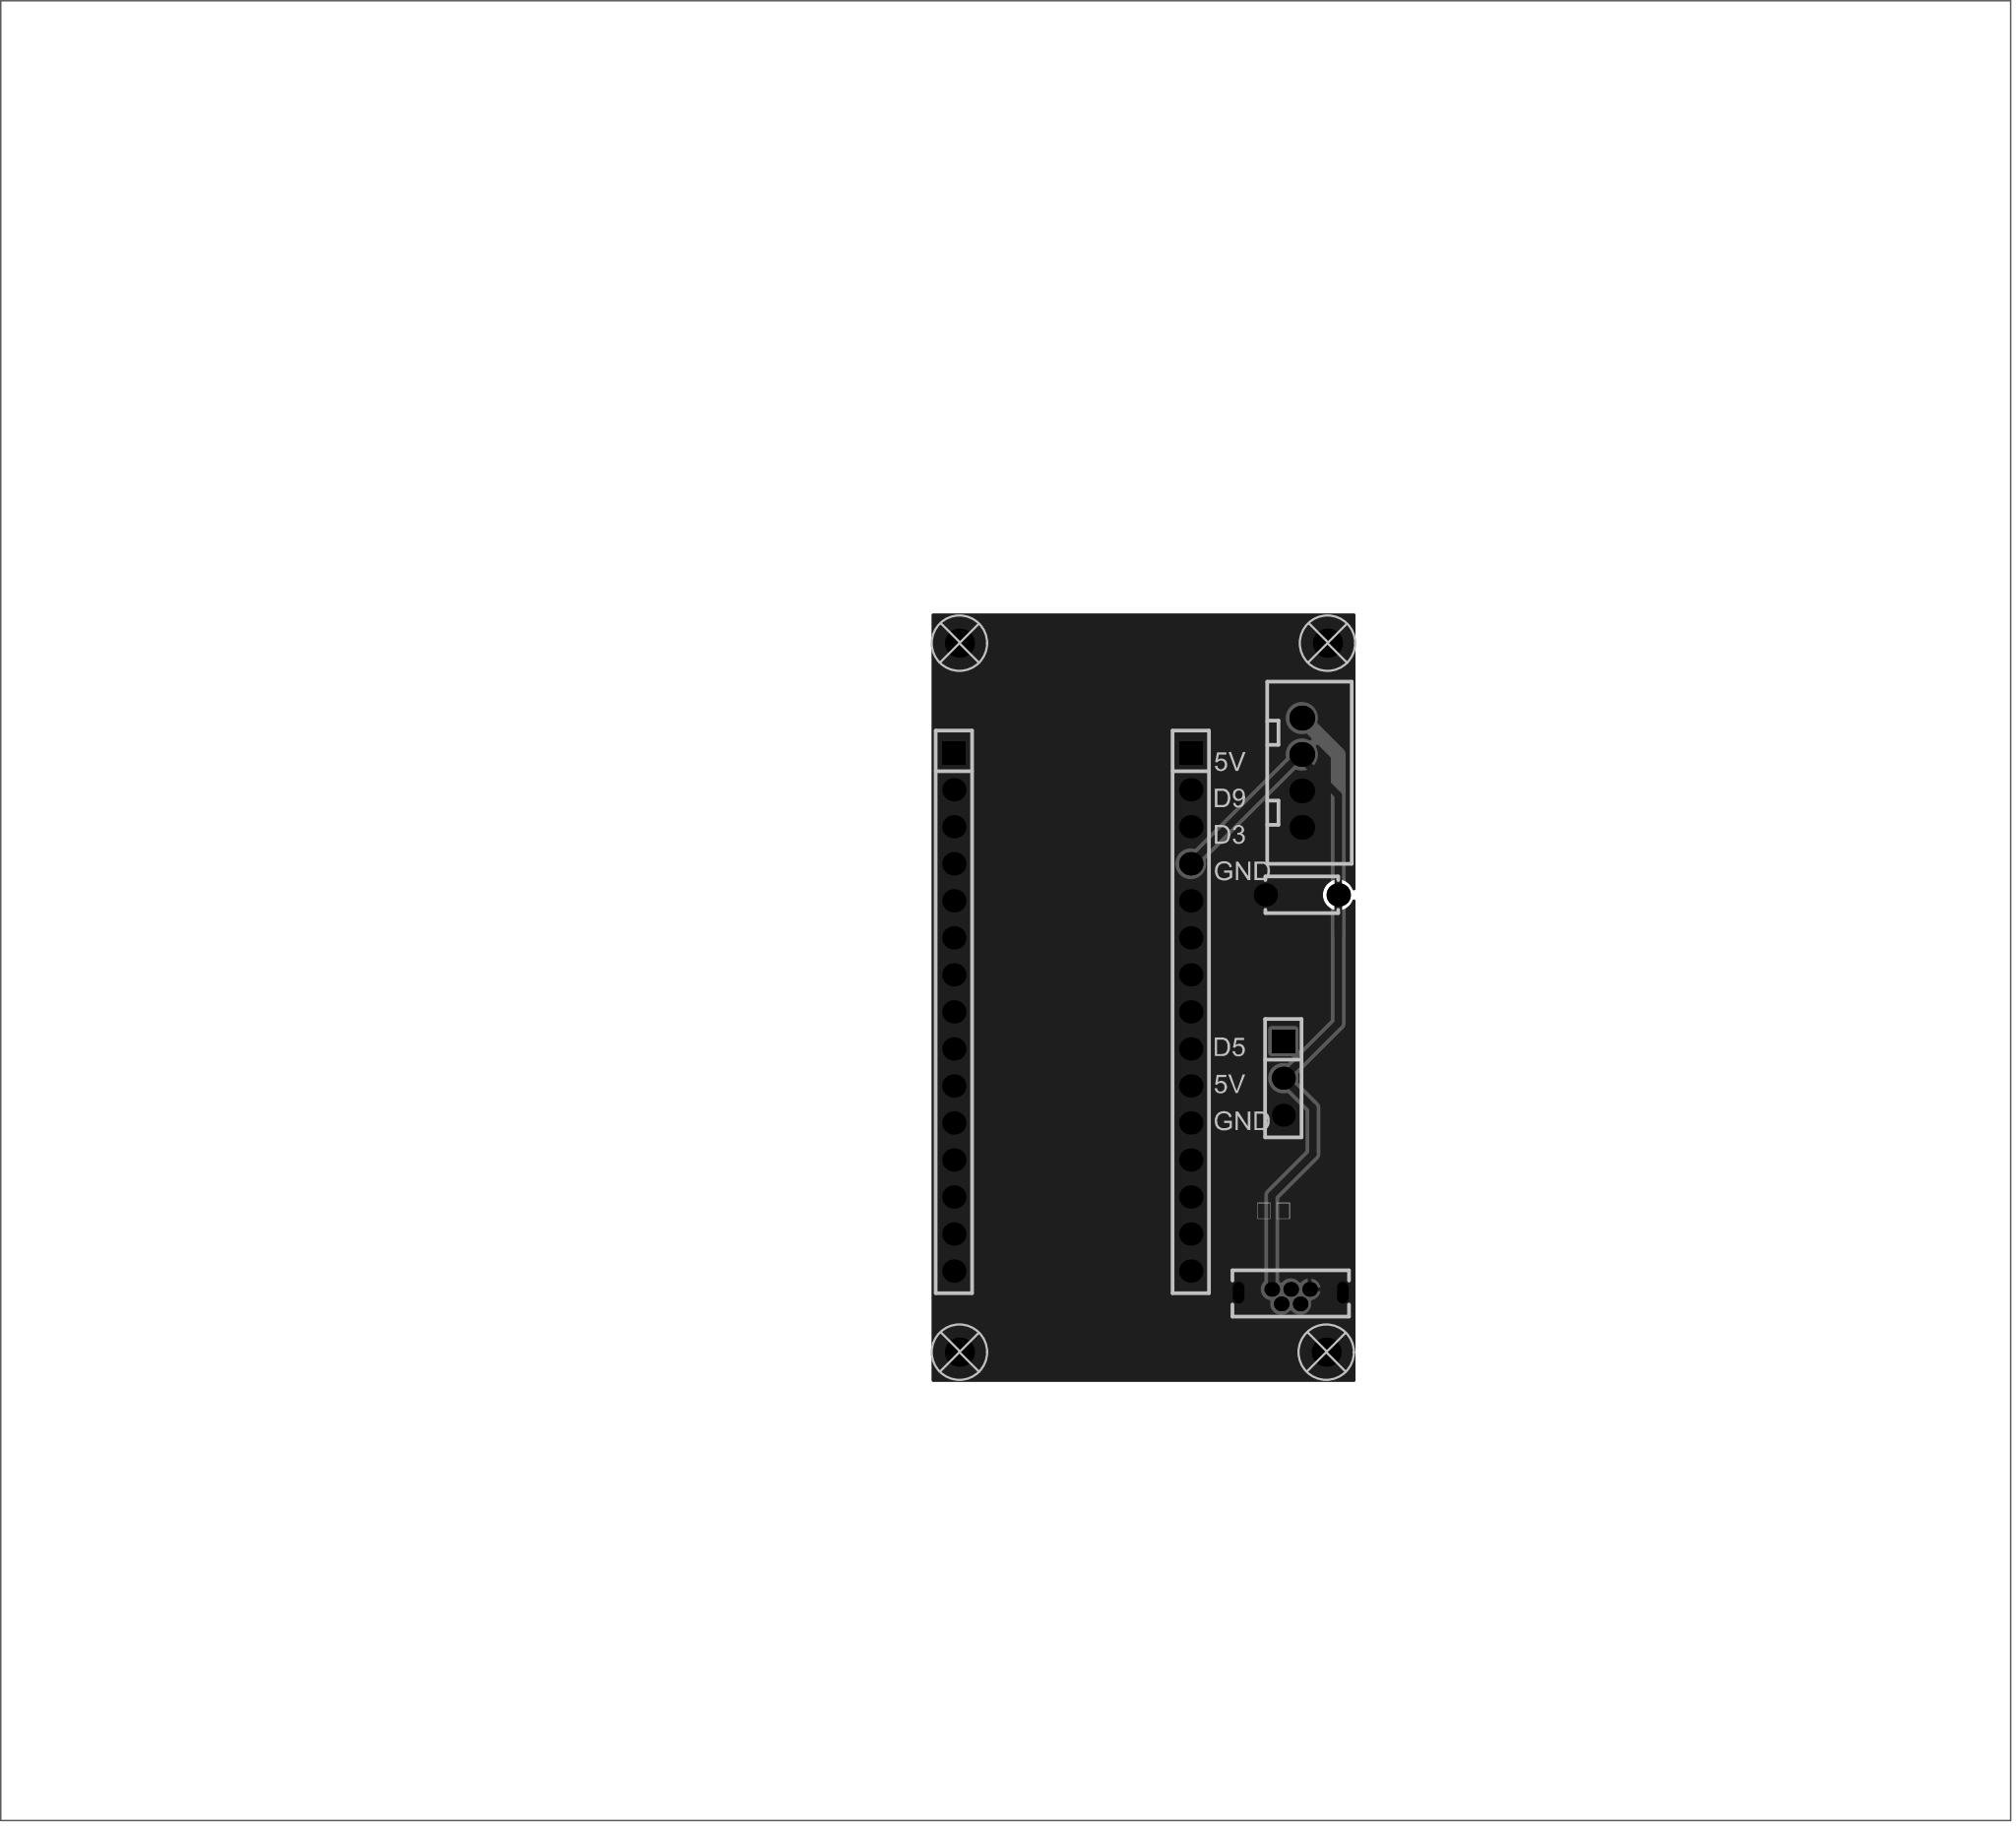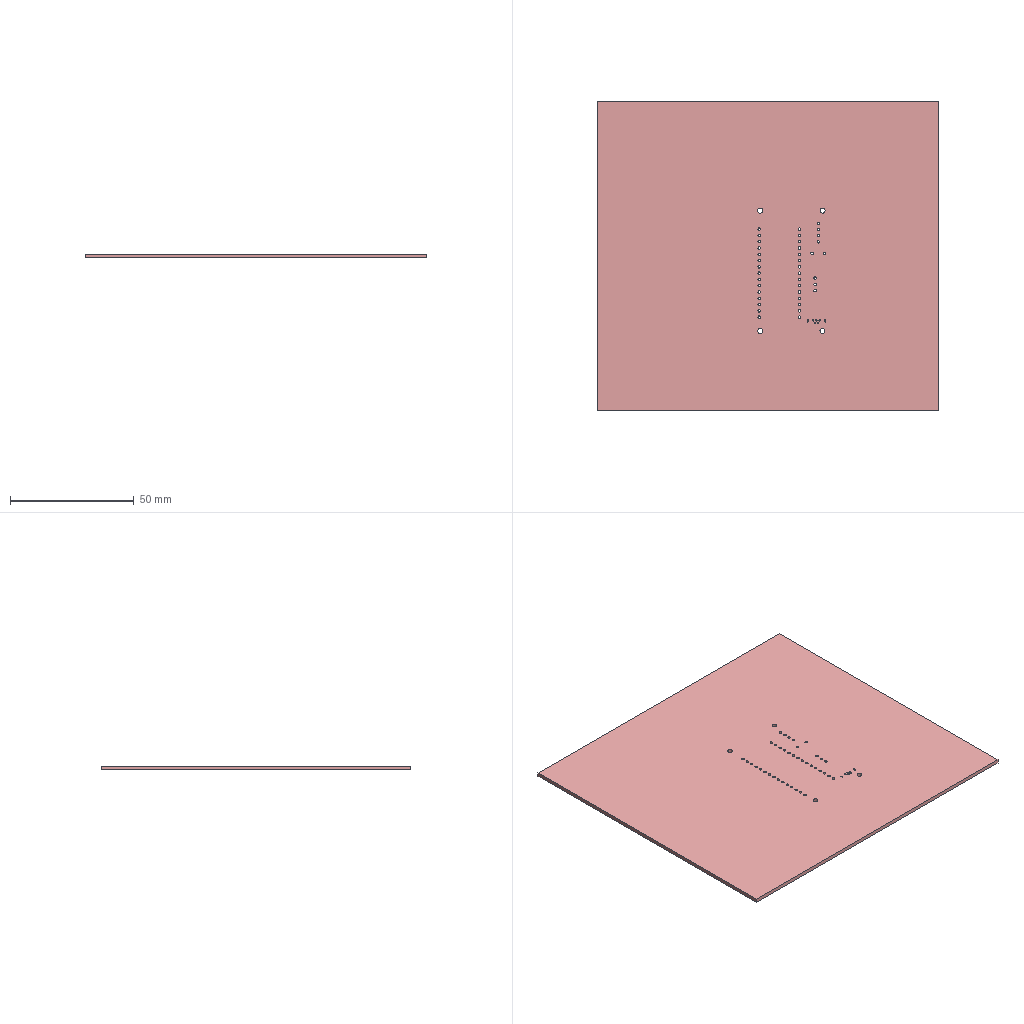Circuit board layout | Altium Designer | box 137.9 x 124.8 x 1.6 mm
Layer stack:
# Altium Designer layer stack of  (unit mm; dielectric type: 0 none, 1 core, 2 prepreg, 3 surface material)
index,name,kind,layer,copper_thickness_mm,dielectric_type,dielectric_thickness_mm,dielectric_material,dielectric_constant
0,Top Paste Mask Layer,other,,,,,,
1,Top Silkscreen Layer,other,,,,,,
2,Top Solder Mask Layer,dielectric,,,3,0.01,,3.3
3,Top Layer,copper,Top Layer,0.035,,,,
4,Dielectric1,dielectric,,,3,1.51,FR4,4.5
5,Bottom Layer,copper,Bottom Layer,0.035,,,,
6,Bottom Solder Mask Layer,dielectric,,,3,0.01,,3.3
7,Bottom Silkscreen Layer,other,,,,,,
8,Bottom Paste Mask Layer,other,,,,,,
# drill layer pairs: low layer,high layer
drill_pair,Top Layer,Bottom Layer
Part placement:
Designator,Comment,Layer,Footprint,Center-X(mm),Center-Y(mm),Rotation
H5,,TopLayer,HDR-TH_15P-P2.54-V-F-1,135.255,125.325,270
H6,,TopLayer,HDR-TH_15P-P2.54-V-F-1,151.511,125.325,270
H1,,TopLayer,HDR-TH_3P-P2.54-V-F,157.861,120.777,270
U1,XH2.54_4P_直插,TopLayer,CONN-TH_4P-P2.50-XH2.54-4P,159.131,141.732,90
U2,100nF,TopLayer,CAP-TH_L5.0-W2.5-P5.00-D1.0,159.131,133.35,180
USB2,HXMICRO180JB2,TopLayer,MICRO-USB-TH_HXMICRO180JB2,158.369,105.791,0
SCREW1,,TopLayer,M2螺丝,135.636,150.622,0
SCREW2,,TopLayer,M2螺丝,160.893,150.622,0
SCREW3,,TopLayer,M2螺丝,135.636,101.981,0
SCREW4,,TopLayer,M2螺丝,160.805,101.981,0
Pad and via stacks:
# Altium Designer via and pad stacks of  (unit mm). Each distinct definition once, with the count of objects using it.
# via: kind,start_layer,end_layer,hole_mm,diameter_mm,mode(0 simple;1 top-mid-bottom;2 full stack),diameter_per_layer,count,example_net
# pad: kind,layer,hole_mm,hole_type(0 round;1 square;2 slot),plating,top_size,top_shape(1 round;2 rect;3 octagon;9 rounded rect),mid_size,bottom_size,mode,footprint,size_per_layer,count,example
pad,Multi-Layer,1,0,plated,1.6x1.6,1,1.6x1.6,1.6x1.6,0,HDR-TH_15P-P2.54-V-F-1,,28,H5.15
pad,Multi-Layer,1,0,plated,1.6x1.575,2,1.6x1.575,1.6x1.575,0,HDR-TH_15P-P2.54-V-F-1,,2,H5.1
pad,Multi-Layer,1.02,0,plated,1.575x1.575,1,1.575x1.575,1.575x1.575,0,HDR-TH_3P-P2.54-V-F,,2,H1.3
pad,Multi-Layer,1.02,0,plated,1.575x1.575,2,1.575x1.575,1.575x1.575,0,HDR-TH_3P-P2.54-V-F,,1,H1.1
pad,Multi-Layer,1.05,0,plated,1.7x1.7,1,1.7x1.7,1.7x1.7,0,CONN-TH_4P-P2.50-XH2.54-4P,,4,U1.1
pad,Multi-Layer,1,0,plated,1.6x1.6,1,1.6x1.6,1.6x1.6,0,CAP-TH_L5.0-W2.5-P5.00-D1.0,,2,U2.1
pad,Multi-Layer,0.6,0,plated,1x1,1,1x1,1x1,0,MICRO-USB-TH_HXMICRO180JB2,,5,USB2.1
pad,Multi-Layer,0.4,2,plated,0.8x1.5,1,0.8x1.5,0.8x1.5,0,MICRO-USB-TH_HXMICRO180JB2,,2,USB2.6
pad,Multi-Layer,2,0,plated,2x2,1,2x2,2x2,0,M2\u00C2\u00DD\u00CB\u00BF,,4,SCREW1.1
Copper pours:
name,layer,net,type(0 solid;1 hatched;2 none)
Bottom Layer-GND,Bottom Layer,GND,0
Top Layer-GND,Top Layer,GND,0
Design rules, without the lines most boards share:
# Altium Designer design rules of  (exported by Altium Designer, unit mm)
# columns: name | kind | enabled | priority | scope1 | scope2 | descriptor | typed fields (field=value)
Copper_copperRegion_copperThickness1oz | 0 | disabled | 4 | All | All | Clearance Constraint (Gap=5.984mil) (Disabled)(All),(All) | gap=0.152
Copper_copperRegion_copperThickness1oz_1 | 63 | disabled | 4 | All | All | Board Clearance Constraint (Gap=0mil) (Disabled)(All) |
Copper_copperRegion_Copper_copperRegion | 0 | disabled | 5 | All | All | Clearance Constraint (Gap=5.984mil) (Disabled)(All),(All) | gap=0.152
Copper_copperRegion_Copper_copperRegion_1 | 63 | disabled | 5 | All | All | Board Clearance Constraint (Gap=0mil) (Disabled)(All) |
copperThickness1oz | 0 | enabled | 6 | All | All | Clearance Constraint (Gap=5.984mil) (All),(All) | gap=0.152
copperThickness1oz_1 | 63 | enabled | 6 | All | All | Board Clearance Constraint (Gap=0mil) (All) |
copperRegion_copperThickness1oz | 20 | disabled | 1 | All | All | Polygon Connect Rule(Relief Connect )(Conductor Width=10mil) (Relief Angle=90 Angle) (Entries=4) (Air Gap Width=10mil) (Disabled)(All),(All) | connect_style(0=relief,1=direct,2=none)=0 relief_conductor_width=0.254 relief_entries=4
copperRegion_Copper_copperRegion | 20 | disabled | 2 | All | All | Polygon Connect Rule(Relief Connect )(Conductor Width=10mil) (Relief Angle=90 Angle) (Entries=4) (Air Gap Width=10mil) (Disabled)(All),(All) | connect_style(0=relief,1=direct,2=none)=0 relief_conductor_width=0.254 relief_entries=4
copperRegion | 20 | enabled | 3 | All | All | Polygon Connect Rule(Relief Connect )(Conductor Width=10mil) (Relief Angle=90 Angle) (Entries=4) (Air Gap Width=10mil) (All),(All) | connect_style(0=relief,1=direct,2=none)=0 relief_conductor_width=0.254 relief_entries=4